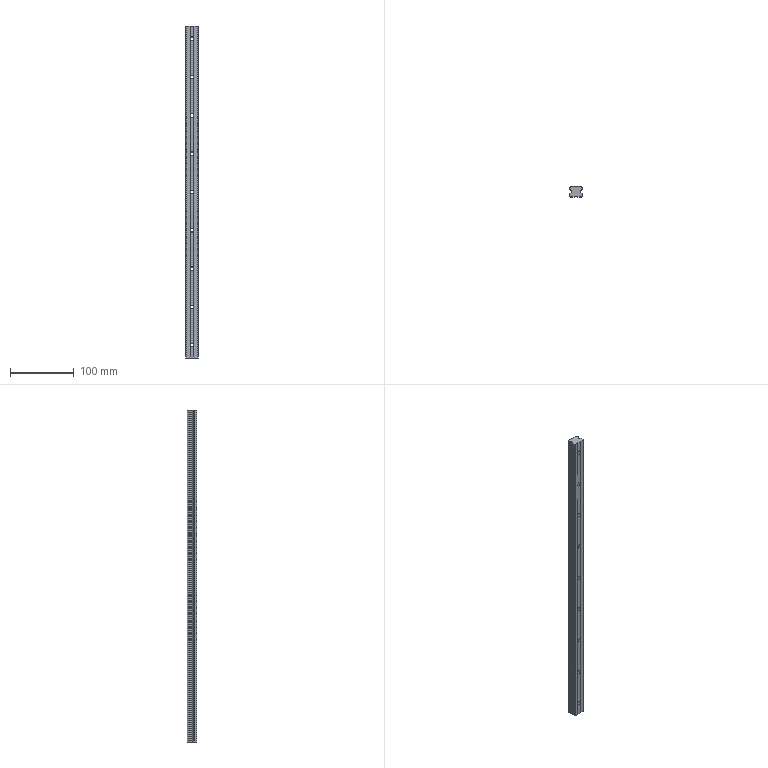Part | NX | features BREP 1 | 1 solid | 99 faces | box 20 x 15.5 x 520 mm | volume 139067 mm3 | cylinder 53 | plane 46 | commonest cylinder face diameters 5.5 x12 10 x12 6 x6 9.5 x6 0.6 x5 2 x5